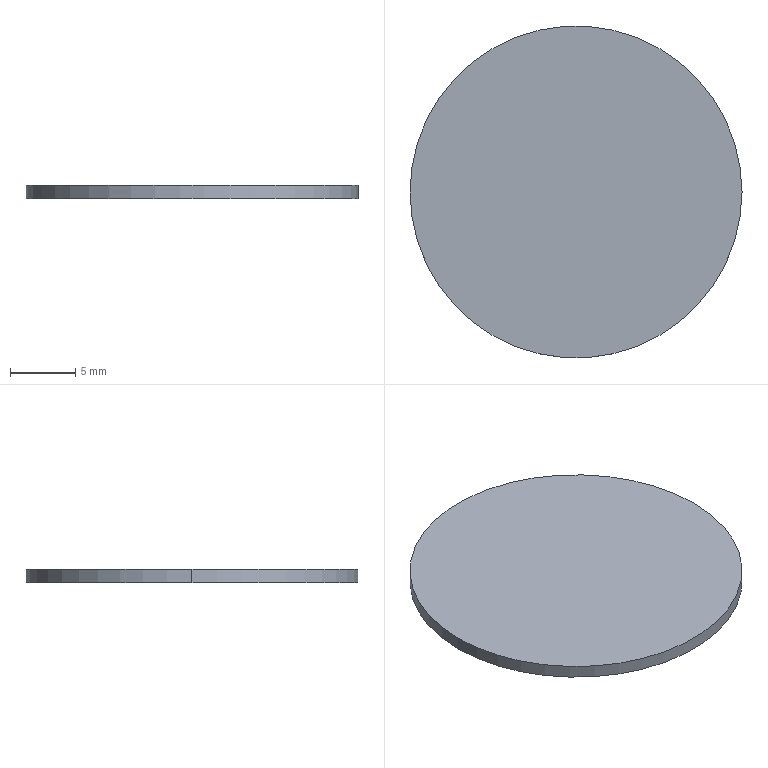Part | SolidWorks | features Extrusion 1 | 1 solid | 4 faces | box 25.4 x 25.4 x 1 mm | volume 506.707 mm3 | cylinder 2 | plane 2 | commonest cylinder face diameters 25.4 x2
STEP:
#1=CARTESIAN_POINT('',(40.9,-28.2,1.));
#2=VERTEX_POINT('',#1);
#3=CARTESIAN_POINT('',(15.5,-28.2,1.));
#4=VERTEX_POINT('',#3);
#5=CARTESIAN_POINT('',(28.2,-28.2,1.));
#6=DIRECTION('',(0.,0.,1.));
#7=DIRECTION('',(1.,0.,0.));
#8=AXIS2_PLACEMENT_3D('',#5,#6,#7);
#9=CIRCLE('',#8,12.7);
#10=EDGE_CURVE('',#2,#4,#9,.T.);
#11=ORIENTED_EDGE('',*,*,#10,.F.);
#12=CARTESIAN_POINT('',(40.9,-28.2,0.));
#13=VERTEX_POINT('',#12);
#14=CARTESIAN_POINT('',(40.9,-28.2,1.));
#15=DIRECTION('',(0.,0.,-1.));
#16=VECTOR('',#15,1000.);
#17=LINE('',#14,#16);
#18=EDGE_CURVE('',#2,#13,#17,.T.);
#19=ORIENTED_EDGE('',*,*,#18,.T.);
#20=CARTESIAN_POINT('',(15.5,-28.2,0.));
#21=VERTEX_POINT('',#20);
#22=CARTESIAN_POINT('',(28.2,-28.2,0.));
#23=DIRECTION('',(0.,0.,1.));
#24=DIRECTION('',(1.,0.,0.));
#25=AXIS2_PLACEMENT_3D('',#22,#23,#24);
#26=CIRCLE('',#25,12.7);
#27=EDGE_CURVE('',#13,#21,#26,.T.);
#28=ORIENTED_EDGE('',*,*,#27,.T.);
#29=CARTESIAN_POINT('',(15.5,-28.2,1.));
#30=DIRECTION('',(0.,0.,-1.));
#31=VECTOR('',#30,1000.);
#32=LINE('',#29,#31);
#33=EDGE_CURVE('',#4,#21,#32,.T.);
#34=ORIENTED_EDGE('',*,*,#33,.F.);
#35=EDGE_LOOP('',(#11,#19,#28,#34));
#36=FACE_OUTER_BOUND('',#35,.T.);
#37=CARTESIAN_POINT('',(28.2,-28.2,1.));
#38=DIRECTION('',(0.,0.,-1.));
#39=DIRECTION('',(-1.,0.,0.));
#40=AXIS2_PLACEMENT_3D('',#37,#38,#39);
#41=CYLINDRICAL_SURFACE('',#40,12.7);
#42=ADVANCED_FACE('',(#36),#41,.T.);
#43=ORIENTED_EDGE('',*,*,#18,.F.);
#44=CARTESIAN_POINT('',(28.2,-28.2,1.));
#45=DIRECTION('',(0.,0.,1.));
#46=DIRECTION('',(1.,0.,0.));
#47=AXIS2_PLACEMENT_3D('',#44,#45,#46);
#48=CIRCLE('',#47,12.7);
#49=EDGE_CURVE('',#4,#2,#48,.T.);
#50=ORIENTED_EDGE('',*,*,#49,.F.);
#51=ORIENTED_EDGE('',*,*,#33,.T.);
#52=CARTESIAN_POINT('',(28.2,-28.2,0.));
#53=DIRECTION('',(0.,0.,1.));
#54=DIRECTION('',(1.,0.,0.));
#55=AXIS2_PLACEMENT_3D('',#52,#53,#54);
#56=CIRCLE('',#55,12.7);
#57=EDGE_CURVE('',#21,#13,#56,.T.);
#58=ORIENTED_EDGE('',*,*,#57,.T.);
#59=EDGE_LOOP('',(#43,#50,#51,#58));
#60=FACE_OUTER_BOUND('',#59,.T.);
#61=CARTESIAN_POINT('',(28.2,-28.2,1.));
#62=DIRECTION('',(0.,0.,-1.));
#63=DIRECTION('',(-1.,0.,0.));
#64=AXIS2_PLACEMENT_3D('',#61,#62,#63);
#65=CYLINDRICAL_SURFACE('',#64,12.7);
#66=ADVANCED_FACE('',(#60),#65,.T.);
#67=ORIENTED_EDGE('',*,*,#49,.T.);
#68=ORIENTED_EDGE('',*,*,#10,.T.);
#69=EDGE_LOOP('',(#67,#68));
#70=FACE_OUTER_BOUND('',#69,.T.);
#71=CARTESIAN_POINT('',(28.2,-28.2,1.));
#72=DIRECTION('',(0.,0.,1.));
#73=DIRECTION('',(1.,0.,0.));
#74=AXIS2_PLACEMENT_3D('',#71,#72,#73);
#75=PLANE('',#74);
#76=ADVANCED_FACE('',(#70),#75,.T.);
#77=ORIENTED_EDGE('',*,*,#57,.F.);
#78=ORIENTED_EDGE('',*,*,#27,.F.);
#79=EDGE_LOOP('',(#77,#78));
#80=FACE_OUTER_BOUND('',#79,.T.);
#81=CARTESIAN_POINT('',(28.2,-28.2,0.));
#82=DIRECTION('',(0.,0.,1.));
#83=DIRECTION('',(1.,0.,0.));
#84=AXIS2_PLACEMENT_3D('',#81,#82,#83);
#85=PLANE('',#84);
#86=ADVANCED_FACE('',(#80),#85,.F.);
#87=CLOSED_SHELL('',(#42,#66,#76,#86));
#88=MANIFOLD_SOLID_BREP('',#87);
#89=CARTESIAN_POINT('',(0.,0.,0.));
#90=DIRECTION('',(0.,0.,1.));
#91=DIRECTION('',(1.,0.,0.));
#92=AXIS2_PLACEMENT_3D('',#89,#90,#91);
#93=(LENGTH_UNIT()NAMED_UNIT(*)SI_UNIT(.MILLI.,.METRE.));
#94=UNCERTAINTY_MEASURE_WITH_UNIT(LENGTH_MEASURE(0.00001),#93,'','');
#95=(NAMED_UNIT(*)PLANE_ANGLE_UNIT()SI_UNIT($,.RADIAN.));
#96=(NAMED_UNIT(*)SI_UNIT($,.STERADIAN.)SOLID_ANGLE_UNIT());
#97=(GEOMETRIC_REPRESENTATION_CONTEXT(3)GLOBAL_UNCERTAINTY_ASSIGNED_CONTEXT((#94))GLOBAL_UNIT_ASSIGNED_CONTEXT((#93,#95,#96))REPRESENTATION_CONTEXT('',''));
#98=ADVANCED_BREP_SHAPE_REPRESENTATION('',(#88,#92),#97);